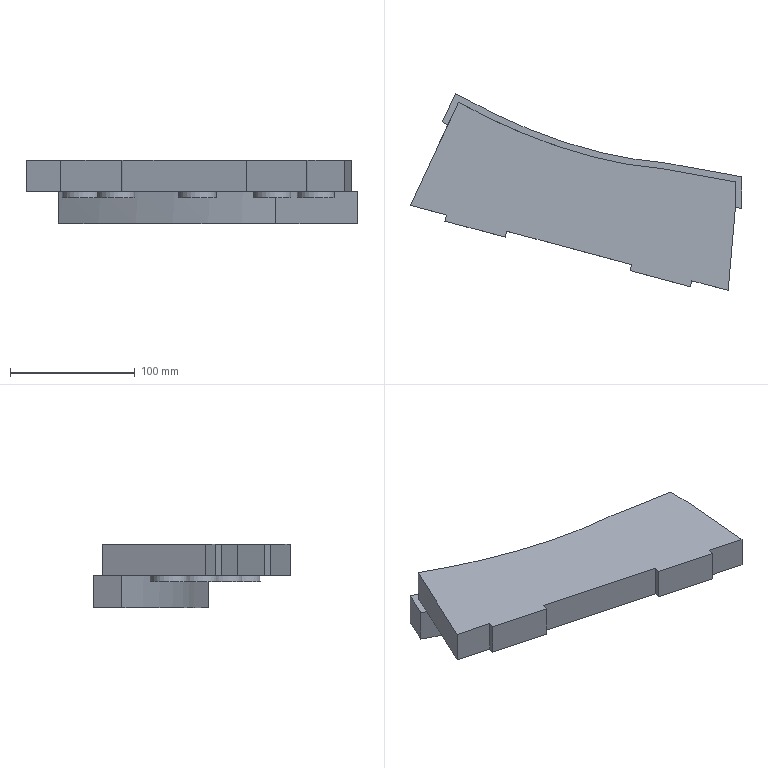Part | NX | features solid 2 | 1 solid | 34 faces | box 265.53 x 157.942 x 51 mm | volume 690173 mm3 | plane 23 | spline 6 | cylinder 5 | commonest cylinder face diameters 30 x5
STEP:
#1=CARTESIAN_POINT('',(-548.514,-260.214,20.));
#2=VERTEX_POINT('',#1);
#3=CARTESIAN_POINT('',(-533.514,-260.214,20.));
#4=DIRECTION('',(0.,0.,-1.));
#5=DIRECTION('',(-1.,0.,0.));
#6=AXIS2_PLACEMENT_3D('',#3,#4,#5);
#7=CIRCLE('',#6,15.);
#8=EDGE_CURVE('',#2,#2,#7,.T.);
#9=ORIENTED_EDGE('',*,*,#8,.T.);
#10=EDGE_LOOP('',(#9));
#11=FACE_BOUND('',#10,.T.);
#12=CARTESIAN_POINT('',(-520.524,-252.714,15.));
#13=VERTEX_POINT('',#12);
#14=CARTESIAN_POINT('',(-533.514,-260.214,15.));
#15=DIRECTION('',(0.,0.,-1.));
#16=DIRECTION('',(0.866,0.5,0.));
#17=AXIS2_PLACEMENT_3D('',#14,#15,#16);
#18=CIRCLE('',#17,15.);
#19=EDGE_CURVE('',#13,#13,#18,.T.);
#20=ORIENTED_EDGE('',*,*,#19,.F.);
#21=EDGE_LOOP('',(#20));
#22=FACE_BOUND('',#21,.T.);
#23=CARTESIAN_POINT('',(-533.514,-260.214,20.));
#24=DIRECTION('',(0.,0.,-1.));
#25=DIRECTION('',(-0.866,-0.5,0.));
#26=AXIS2_PLACEMENT_3D('',#23,#24,#25);
#27=CYLINDRICAL_SURFACE('',#26,15.);
#28=ADVANCED_FACE('',(#11,#22),#27,.T.);
#29=CARTESIAN_POINT('',(-613.514,-240.214,20.));
#30=VERTEX_POINT('',#29);
#31=CARTESIAN_POINT('',(-598.514,-240.214,20.));
#32=DIRECTION('',(0.,0.,-1.));
#33=DIRECTION('',(-1.,0.,0.));
#34=AXIS2_PLACEMENT_3D('',#31,#32,#33);
#35=CIRCLE('',#34,15.);
#36=EDGE_CURVE('',#30,#30,#35,.T.);
#37=ORIENTED_EDGE('',*,*,#36,.T.);
#38=EDGE_LOOP('',(#37));
#39=FACE_BOUND('',#38,.T.);
#40=CARTESIAN_POINT('',(-583.514,-240.214,15.));
#41=VERTEX_POINT('',#40);
#42=CARTESIAN_POINT('',(-598.514,-240.214,15.));
#43=DIRECTION('',(0.,0.,1.));
#44=DIRECTION('',(1.,0.,0.));
#45=AXIS2_PLACEMENT_3D('',#42,#43,#44);
#46=CIRCLE('',#45,15.);
#47=EDGE_CURVE('',#41,#41,#46,.T.);
#48=ORIENTED_EDGE('',*,*,#47,.T.);
#49=EDGE_LOOP('',(#48));
#50=FACE_BOUND('',#49,.T.);
#51=CARTESIAN_POINT('',(-598.514,-240.214,20.));
#52=DIRECTION('',(0.,0.,-1.));
#53=DIRECTION('',(-0.866,-0.5,0.));
#54=AXIS2_PLACEMENT_3D('',#51,#52,#53);
#55=CYLINDRICAL_SURFACE('',#54,15.);
#56=ADVANCED_FACE('',(#39,#50),#55,.T.);
#57=CARTESIAN_POINT('',(-594.55,-271.507,45.));
#58=VERTEX_POINT('',#57);
#59=CARTESIAN_POINT('',(-642.847,-258.566,45.));
#60=VERTEX_POINT('',#59);
#61=CARTESIAN_POINT('',(-576.068,-276.459,45.));
#62=DIRECTION('',(-0.9659,0.2588,0.));
#63=VECTOR('',#62,1000.);
#64=LINE('',#61,#63);
#65=EDGE_CURVE('',#58,#60,#64,.T.);
#66=ORIENTED_EDGE('',*,*,#65,.T.);
#67=CARTESIAN_POINT('',(-642.847,-258.566,20.));
#68=VERTEX_POINT('',#67);
#69=CARTESIAN_POINT('',(-642.847,-258.566,45.));
#70=DIRECTION('',(0.,0.,-1.));
#71=VECTOR('',#70,1000.);
#72=LINE('',#69,#71);
#73=EDGE_CURVE('',#60,#68,#72,.T.);
#74=ORIENTED_EDGE('',*,*,#73,.T.);
#75=CARTESIAN_POINT('',(-594.55,-271.507,20.));
#76=VERTEX_POINT('',#75);
#77=CARTESIAN_POINT('',(-455.717,-308.707,20.));
#78=DIRECTION('',(-0.9659,0.2588,0.));
#79=VECTOR('',#78,1000.);
#80=LINE('',#77,#79);
#81=EDGE_CURVE('',#76,#68,#80,.T.);
#82=ORIENTED_EDGE('',*,*,#81,.F.);
#83=CARTESIAN_POINT('',(-594.55,-271.507,45.));
#84=DIRECTION('',(0.,0.,-1.));
#85=VECTOR('',#84,1000.);
#86=LINE('',#83,#85);
#87=EDGE_CURVE('',#58,#76,#86,.T.);
#88=ORIENTED_EDGE('',*,*,#87,.F.);
#89=EDGE_LOOP('',(#66,#74,#82,#88));
#90=FACE_BOUND('',#89,.T.);
#91=CARTESIAN_POINT('',(-401.118,-323.337,45.));
#92=DIRECTION('',(-0.2588,-0.9659,0.));
#93=DIRECTION('',(0.9659,-0.2588,0.));
#94=AXIS2_PLACEMENT_3D('',#91,#92,#93);
#95=PLANE('',#94);
#96=ADVANCED_FACE('',(#90),#95,.T.);
#97=CARTESIAN_POINT('',(-593.256,-266.677,45.));
#98=VERTEX_POINT('',#97);
#99=CARTESIAN_POINT('',(-593.256,-266.677,20.));
#100=VERTEX_POINT('',#99);
#101=CARTESIAN_POINT('',(-593.256,-266.677,45.));
#102=DIRECTION('',(0.,0.,-1.));
#103=VECTOR('',#102,1000.);
#104=LINE('',#101,#103);
#105=EDGE_CURVE('',#98,#100,#104,.T.);
#106=ORIENTED_EDGE('',*,*,#105,.F.);
#107=CARTESIAN_POINT('',(-594.55,-271.507,45.));
#108=DIRECTION('',(0.2588,0.9659,0.));
#109=VECTOR('',#108,1000.);
#110=LINE('',#107,#109);
#111=EDGE_CURVE('',#58,#98,#110,.T.);
#112=ORIENTED_EDGE('',*,*,#111,.F.);
#113=ORIENTED_EDGE('',*,*,#87,.T.);
#114=CARTESIAN_POINT('',(-594.55,-271.507,20.));
#115=DIRECTION('',(0.2588,0.9659,0.));
#116=VECTOR('',#115,1000.);
#117=LINE('',#114,#116);
#118=EDGE_CURVE('',#76,#100,#117,.T.);
#119=ORIENTED_EDGE('',*,*,#118,.T.);
#120=EDGE_LOOP('',(#106,#112,#113,#119));
#121=FACE_BOUND('',#120,.T.);
#122=CARTESIAN_POINT('',(-594.55,-271.507,45.));
#123=DIRECTION('',(0.9659,-0.2588,0.));
#124=DIRECTION('',(0.2588,0.9659,0.));
#125=AXIS2_PLACEMENT_3D('',#122,#123,#124);
#126=PLANE('',#125);
#127=ADVANCED_FACE('',(#121),#126,.T.);
#128=CARTESIAN_POINT('',(-641.553,-253.736,45.));
#129=VERTEX_POINT('',#128);
#130=CARTESIAN_POINT('',(-670.53,-245.972,45.));
#131=VERTEX_POINT('',#130);
#132=CARTESIAN_POINT('',(-574.774,-271.63,45.));
#133=DIRECTION('',(-0.9659,0.2588,0.));
#134=VECTOR('',#133,1000.);
#135=LINE('',#132,#134);
#136=EDGE_CURVE('',#129,#131,#135,.T.);
#137=ORIENTED_EDGE('',*,*,#136,.T.);
#138=CARTESIAN_POINT('',(-670.53,-245.972,20.));
#139=VERTEX_POINT('',#138);
#140=CARTESIAN_POINT('',(-670.53,-245.972,45.));
#141=DIRECTION('',(0.,0.,-1.));
#142=VECTOR('',#141,1000.);
#143=LINE('',#140,#142);
#144=EDGE_CURVE('',#131,#139,#143,.T.);
#145=ORIENTED_EDGE('',*,*,#144,.T.);
#146=CARTESIAN_POINT('',(-641.553,-253.736,20.));
#147=VERTEX_POINT('',#146);
#148=CARTESIAN_POINT('',(-454.423,-303.878,20.));
#149=DIRECTION('',(-0.9659,0.2588,0.));
#150=VECTOR('',#149,1000.);
#151=LINE('',#148,#150);
#152=EDGE_CURVE('',#147,#139,#151,.T.);
#153=ORIENTED_EDGE('',*,*,#152,.F.);
#154=CARTESIAN_POINT('',(-641.553,-253.736,45.));
#155=DIRECTION('',(0.,0.,-1.));
#156=VECTOR('',#155,1000.);
#157=LINE('',#154,#156);
#158=EDGE_CURVE('',#129,#147,#157,.T.);
#159=ORIENTED_EDGE('',*,*,#158,.F.);
#160=EDGE_LOOP('',(#137,#145,#153,#159));
#161=FACE_BOUND('',#160,.T.);
#162=CARTESIAN_POINT('',(-399.824,-318.507,45.));
#163=DIRECTION('',(-0.2588,-0.9659,0.));
#164=DIRECTION('',(0.9659,-0.2588,0.));
#165=AXIS2_PLACEMENT_3D('',#162,#163,#164);
#166=PLANE('',#165);
#167=ADVANCED_FACE('',(#161),#166,.T.);
#168=ORIENTED_EDGE('',*,*,#158,.T.);
#169=CARTESIAN_POINT('',(-642.847,-258.566,20.));
#170=DIRECTION('',(0.2588,0.9659,0.));
#171=VECTOR('',#170,1000.);
#172=LINE('',#169,#171);
#173=EDGE_CURVE('',#68,#147,#172,.T.);
#174=ORIENTED_EDGE('',*,*,#173,.F.);
#175=ORIENTED_EDGE('',*,*,#73,.F.);
#176=CARTESIAN_POINT('',(-642.847,-258.566,45.));
#177=DIRECTION('',(0.2588,0.9659,0.));
#178=VECTOR('',#177,1000.);
#179=LINE('',#176,#178);
#180=EDGE_CURVE('',#60,#129,#179,.T.);
#181=ORIENTED_EDGE('',*,*,#180,.T.);
#182=EDGE_LOOP('',(#168,#174,#175,#181));
#183=FACE_BOUND('',#182,.T.);
#184=CARTESIAN_POINT('',(-642.847,-258.566,45.));
#185=DIRECTION('',(0.9659,-0.2588,0.));
#186=DIRECTION('',(0.2588,0.9659,0.));
#187=AXIS2_PLACEMENT_3D('',#184,#185,#186);
#188=PLANE('',#187);
#189=ADVANCED_FACE('',(#183),#188,.F.);
#190=CARTESIAN_POINT('',(-425.524,-262.714,15.));
#191=VERTEX_POINT('',#190);
#192=CARTESIAN_POINT('',(-438.514,-270.214,15.));
#193=DIRECTION('',(0.,0.,-1.));
#194=DIRECTION('',(0.866,0.5,0.));
#195=AXIS2_PLACEMENT_3D('',#192,#193,#194);
#196=CIRCLE('',#195,15.);
#197=EDGE_CURVE('',#191,#191,#196,.T.);
#198=ORIENTED_EDGE('',*,*,#197,.F.);
#199=EDGE_LOOP('',(#198));
#200=FACE_BOUND('',#199,.T.);
#201=CARTESIAN_POINT('',(-453.514,-270.214,20.));
#202=VERTEX_POINT('',#201);
#203=CARTESIAN_POINT('',(-438.514,-270.214,20.));
#204=DIRECTION('',(0.,0.,-1.));
#205=DIRECTION('',(-1.,0.,0.));
#206=AXIS2_PLACEMENT_3D('',#203,#204,#205);
#207=CIRCLE('',#206,15.);
#208=EDGE_CURVE('',#202,#202,#207,.T.);
#209=ORIENTED_EDGE('',*,*,#208,.T.);
#210=EDGE_LOOP('',(#209));
#211=FACE_BOUND('',#210,.T.);
#212=CARTESIAN_POINT('',(-438.514,-270.214,20.));
#213=DIRECTION('',(0.,0.,-1.));
#214=DIRECTION('',(-0.866,-0.5,0.));
#215=AXIS2_PLACEMENT_3D('',#212,#213,#214);
#216=CYLINDRICAL_SURFACE('',#215,15.);
#217=ADVANCED_FACE('',(#200,#211),#216,.T.);
#218=CARTESIAN_POINT('',(-415.836,-314.217,20.));
#219=VERTEX_POINT('',#218);
#220=CARTESIAN_POINT('',(-410.,-247.512,20.));
#221=VERTEX_POINT('',#220);
#222=CARTESIAN_POINT('',(-409.784,-245.039,20.));
#223=DIRECTION('',(0.08716,0.9962,0.));
#224=VECTOR('',#223,1000.);
#225=LINE('',#222,#224);
#226=EDGE_CURVE('',#219,#221,#225,.T.);
#227=ORIENTED_EDGE('',*,*,#226,.T.);
#228=CARTESIAN_POINT('',(-410.,-247.512,45.));
#229=VERTEX_POINT('',#228);
#230=CARTESIAN_POINT('',(-410.,-247.512,20.));
#231=DIRECTION('',(0.,0.,1.));
#232=VECTOR('',#231,1000.);
#233=LINE('',#230,#232);
#234=EDGE_CURVE('',#221,#229,#233,.T.);
#235=ORIENTED_EDGE('',*,*,#234,.T.);
#236=CARTESIAN_POINT('',(-415.836,-314.217,45.));
#237=VERTEX_POINT('',#236);
#238=CARTESIAN_POINT('',(-406.364,-205.947,45.));
#239=DIRECTION('',(0.08716,0.9962,0.));
#240=VECTOR('',#239,1000.);
#241=LINE('',#238,#240);
#242=EDGE_CURVE('',#237,#229,#241,.T.);
#243=ORIENTED_EDGE('',*,*,#242,.F.);
#244=CARTESIAN_POINT('',(-415.836,-314.217,45.));
#245=DIRECTION('',(0.,0.,-1.));
#246=VECTOR('',#245,1000.);
#247=LINE('',#244,#246);
#248=EDGE_CURVE('',#237,#219,#247,.T.);
#249=ORIENTED_EDGE('',*,*,#248,.T.);
#250=EDGE_LOOP('',(#227,#235,#243,#249));
#251=FACE_BOUND('',#250,.T.);
#252=CARTESIAN_POINT('',(-410.,-247.512,26.));
#253=DIRECTION('',(-0.9962,0.08716,0.));
#254=DIRECTION('',(-0.08716,-0.9962,0.));
#255=AXIS2_PLACEMENT_3D('',#252,#253,#254);
#256=PLANE('',#255);
#257=ADVANCED_FACE('',(#251),#256,.F.);
#258=CARTESIAN_POINT('',(-640.447,-181.458,20.));
#259=VERTEX_POINT('',#258);
#260=CARTESIAN_POINT('',(-470.646,-236.588,20.));
#261=VERTEX_POINT('',#260);
#262=CARTESIAN_POINT('',(-640.447,-181.458,20.));
#263=CARTESIAN_POINT('',(-627.329,-188.713,20.));
#264=CARTESIAN_POINT('',(-600.49,-202.118,20.));
#265=CARTESIAN_POINT('',(-558.614,-218.615,20.));
#266=CARTESIAN_POINT('',(-515.266,-230.753,20.));
#267=CARTESIAN_POINT('',(-485.578,-235.315,20.));
#268=CARTESIAN_POINT('',(-470.646,-236.588,20.));
#269=B_SPLINE_CURVE_WITH_KNOTS('',3,(#262,#263,#264,#265,#266,#267,#268),.UNSPECIFIED.,.F.,.F.,(4,1,1,1,4),(0.7368,0.7817,0.8267,0.8717,0.9167),.UNSPECIFIED.);
#270=EDGE_CURVE('',#259,#261,#269,.T.);
#271=ORIENTED_EDGE('',*,*,#270,.F.);
#272=CARTESIAN_POINT('',(-644.823,-179.011,20.));
#273=VERTEX_POINT('',#272);
#274=CARTESIAN_POINT('',(-644.823,-179.011,20.));
#275=CARTESIAN_POINT('',(-643.368,-179.833,20.));
#276=CARTESIAN_POINT('',(-641.909,-180.649,20.));
#277=CARTESIAN_POINT('',(-640.447,-181.458,20.));
#278=B_SPLINE_CURVE_WITH_KNOTS('',3,(#274,#275,#276,#277),.UNSPECIFIED.,.F.,.F.,(4,4),(0.7318,0.7368),.UNSPECIFIED.);
#279=EDGE_CURVE('',#273,#259,#278,.T.);
#280=ORIENTED_EDGE('',*,*,#279,.F.);
#281=CARTESIAN_POINT('',(-644.823,-179.011,-6.));
#282=VERTEX_POINT('',#281);
#283=CARTESIAN_POINT('',(-644.823,-179.011,45.));
#284=DIRECTION('',(0.,0.,-1.));
#285=VECTOR('',#284,1000.);
#286=LINE('',#283,#285);
#287=EDGE_CURVE('',#273,#282,#286,.T.);
#288=ORIENTED_EDGE('',*,*,#287,.T.);
#289=CARTESIAN_POINT('',(-470.646,-236.588,-6.));
#290=VERTEX_POINT('',#289);
#291=CARTESIAN_POINT('',(-644.823,-179.011,-6.));
#292=CARTESIAN_POINT('',(-641.958,-180.631,-6.));
#293=CARTESIAN_POINT('',(-622.134,-191.596,-6.));
#294=CARTESIAN_POINT('',(-584.151,-209.58,-6.));
#295=CARTESIAN_POINT('',(-528.839,-228.144,-6.));
#296=CARTESIAN_POINT('',(-490.07,-234.932,-6.));
#297=CARTESIAN_POINT('',(-470.646,-236.588,-6.));
#298=B_SPLINE_CURVE_WITH_KNOTS('',3,(#291,#292,#293,#294,#295,#296,#297),.UNSPECIFIED.,.F.,.F.,(4,1,1,1,4),(0.,0.04001,0.2754,0.5108,0.7411),.UNSPECIFIED.);
#299=EDGE_CURVE('',#282,#290,#298,.T.);
#300=ORIENTED_EDGE('',*,*,#299,.T.);
#301=CARTESIAN_POINT('',(-470.646,-236.588,45.));
#302=DIRECTION('',(0.,0.,-1.));
#303=VECTOR('',#302,1000.);
#304=LINE('',#301,#303);
#305=EDGE_CURVE('',#261,#290,#304,.T.);
#306=ORIENTED_EDGE('',*,*,#305,.F.);
#307=EDGE_LOOP('',(#271,#280,#288,#300,#306));
#308=FACE_BOUND('',#307,.T.);
#309=CARTESIAN_POINT('',(-644.823,-179.011,20.));
#310=CARTESIAN_POINT('',(-644.823,-179.011,-6.));
#311=CARTESIAN_POINT('',(-631.553,-186.516,20.));
#312=CARTESIAN_POINT('',(-631.553,-186.516,-6.));
#313=CARTESIAN_POINT('',(-604.421,-200.366,20.));
#314=CARTESIAN_POINT('',(-604.421,-200.366,-6.));
#315=CARTESIAN_POINT('',(-561.818,-217.552,20.));
#316=CARTESIAN_POINT('',(-561.818,-217.552,-6.));
#317=CARTESIAN_POINT('',(-517.207,-230.394,20.));
#318=CARTESIAN_POINT('',(-517.207,-230.394,-6.));
#319=CARTESIAN_POINT('',(-486.272,-235.255,20.));
#320=CARTESIAN_POINT('',(-486.272,-235.255,-6.));
#321=CARTESIAN_POINT('',(-470.646,-236.588,20.));
#322=CARTESIAN_POINT('',(-470.646,-236.588,-6.));
#323=B_SPLINE_SURFACE_WITH_KNOTS('',3,1,((#309,#310),(#311,#312),(#313,#314),(#315,#316),(#317,#318),(#319,#320),(#321,#322)),.SURF_OF_LINEAR_EXTRUSION.,.F.,.F.,.F.,(4,1,1,1,4),(2,2),(0.,0.1853,0.3706,0.5559,0.7411),(0.,1.),.UNSPECIFIED.);
#324=ADVANCED_FACE('',(#308),#323,.F.);
#325=CARTESIAN_POINT('',(-405.,-248.354,-6.));
#326=VERTEX_POINT('',#325);
#327=CARTESIAN_POINT('',(-470.646,-236.588,-6.));
#328=CARTESIAN_POINT('',(-456.993,-239.107,-6.));
#329=CARTESIAN_POINT('',(-435.255,-243.115,-6.));
#330=CARTESIAN_POINT('',(-413.219,-246.983,-6.));
#331=CARTESIAN_POINT('',(-405.,-248.354,-6.));
#332=B_SPLINE_CURVE_WITH_KNOTS('',3,(#327,#328,#329,#330,#331),.UNSPECIFIED.,.F.,.F.,(4,1,4),(0.7411,0.9039,1.),.UNSPECIFIED.);
#333=EDGE_CURVE('',#290,#326,#332,.T.);
#334=ORIENTED_EDGE('',*,*,#333,.T.);
#335=CARTESIAN_POINT('',(-405.,-248.354,20.));
#336=VERTEX_POINT('',#335);
#337=CARTESIAN_POINT('',(-405.,-248.354,45.));
#338=DIRECTION('',(0.,0.,-1.));
#339=VECTOR('',#338,1000.);
#340=LINE('',#337,#339);
#341=EDGE_CURVE('',#336,#326,#340,.T.);
#342=ORIENTED_EDGE('',*,*,#341,.F.);
#343=CARTESIAN_POINT('',(-470.646,-236.588,20.));
#344=CARTESIAN_POINT('',(-456.993,-239.107,20.));
#345=CARTESIAN_POINT('',(-435.255,-243.115,20.));
#346=CARTESIAN_POINT('',(-413.219,-246.983,20.));
#347=CARTESIAN_POINT('',(-405.,-248.354,20.));
#348=B_SPLINE_CURVE_WITH_KNOTS('',3,(#343,#344,#345,#346,#347),.UNSPECIFIED.,.F.,.F.,(4,1,4),(0.7411,0.9039,1.),.UNSPECIFIED.);
#349=EDGE_CURVE('',#336,#221,#348,.F.);
#350=ORIENTED_EDGE('',*,*,#349,.T.);
#351=CARTESIAN_POINT('',(-470.646,-236.588,20.));
#352=CARTESIAN_POINT('',(-450.446,-240.315,20.));
#353=CARTESIAN_POINT('',(-430.25,-244.067,20.));
#354=CARTESIAN_POINT('',(-410.,-247.512,20.));
#355=B_SPLINE_CURVE_WITH_KNOTS('',3,(#351,#352,#353,#354),.UNSPECIFIED.,.F.,.F.,(4,4),(0.07034,0.132),.UNSPECIFIED.);
#356=EDGE_CURVE('',#261,#221,#355,.T.);
#357=ORIENTED_EDGE('',*,*,#356,.F.);
#358=ORIENTED_EDGE('',*,*,#305,.T.);
#359=EDGE_LOOP('',(#334,#342,#350,#357,#358));
#360=FACE_BOUND('',#359,.T.);
#361=CARTESIAN_POINT('',(-470.646,-236.588,20.));
#362=CARTESIAN_POINT('',(-470.646,-236.588,-6.));
#363=CARTESIAN_POINT('',(-448.934,-240.594,20.));
#364=CARTESIAN_POINT('',(-448.934,-240.594,-6.));
#365=CARTESIAN_POINT('',(-427.143,-244.66,20.));
#366=CARTESIAN_POINT('',(-427.143,-244.66,-6.));
#367=CARTESIAN_POINT('',(-405.,-248.354,20.));
#368=CARTESIAN_POINT('',(-405.,-248.354,-6.));
#369=B_SPLINE_SURFACE_WITH_KNOTS('',3,1,((#361,#362),(#363,#364),(#365,#366),(#367,#368)),.SURF_OF_LINEAR_EXTRUSION.,.F.,.F.,.F.,(4,4),(2,2),(0.7411,1.),(0.,1.),.PIECEWISE_BEZIER_KNOTS.);
#370=ADVANCED_FACE('',(#360),#369,.F.);
#371=CARTESIAN_POINT('',(-613.873,-209.233,15.));
#372=VERTEX_POINT('',#371);
#373=CARTESIAN_POINT('',(-626.864,-216.733,15.));
#374=DIRECTION('',(0.,0.,-1.));
#375=DIRECTION('',(0.866,0.5,0.));
#376=AXIS2_PLACEMENT_3D('',#373,#374,#375);
#377=CIRCLE('',#376,15.);
#378=EDGE_CURVE('',#372,#372,#377,.T.);
#379=ORIENTED_EDGE('',*,*,#378,.F.);
#380=EDGE_LOOP('',(#379));
#381=FACE_BOUND('',#380,.T.);
#382=CARTESIAN_POINT('',(-641.864,-216.733,20.));
#383=VERTEX_POINT('',#382);
#384=CARTESIAN_POINT('',(-626.864,-216.733,20.));
#385=DIRECTION('',(0.,0.,-1.));
#386=DIRECTION('',(-1.,0.,0.));
#387=AXIS2_PLACEMENT_3D('',#384,#385,#386);
#388=CIRCLE('',#387,15.);
#389=EDGE_CURVE('',#383,#383,#388,.T.);
#390=ORIENTED_EDGE('',*,*,#389,.T.);
#391=EDGE_LOOP('',(#390));
#392=FACE_BOUND('',#391,.T.);
#393=CARTESIAN_POINT('',(-626.864,-216.733,20.));
#394=DIRECTION('',(0.,0.,-1.));
#395=DIRECTION('',(-0.866,-0.5,0.));
#396=AXIS2_PLACEMENT_3D('',#393,#394,#395);
#397=CYLINDRICAL_SURFACE('',#396,15.);
#398=ADVANCED_FACE('',(#381,#392),#397,.T.);
#399=CARTESIAN_POINT('',(-488.514,-275.214,20.));
#400=VERTEX_POINT('',#399);
#401=CARTESIAN_POINT('',(-473.514,-275.214,20.));
#402=DIRECTION('',(0.,0.,-1.));
#403=DIRECTION('',(-1.,0.,0.));
#404=AXIS2_PLACEMENT_3D('',#401,#402,#403);
#405=CIRCLE('',#404,15.);
#406=EDGE_CURVE('',#400,#400,#405,.T.);
#407=ORIENTED_EDGE('',*,*,#406,.T.);
#408=EDGE_LOOP('',(#407));
#409=FACE_BOUND('',#408,.T.);
#410=CARTESIAN_POINT('',(-460.524,-267.714,15.));
#411=VERTEX_POINT('',#410);
#412=CARTESIAN_POINT('',(-473.514,-275.214,15.));
#413=DIRECTION('',(0.,0.,-1.));
#414=DIRECTION('',(0.866,0.5,0.));
#415=AXIS2_PLACEMENT_3D('',#412,#413,#414);
#416=CIRCLE('',#415,15.);
#417=EDGE_CURVE('',#411,#411,#416,.T.);
#418=ORIENTED_EDGE('',*,*,#417,.F.);
#419=EDGE_LOOP('',(#418));
#420=FACE_BOUND('',#419,.T.);
#421=CARTESIAN_POINT('',(-473.514,-275.214,20.));
#422=DIRECTION('',(0.,0.,-1.));
#423=DIRECTION('',(-0.866,-0.5,0.));
#424=AXIS2_PLACEMENT_3D('',#421,#422,#423);
#425=CYLINDRICAL_SURFACE('',#424,15.);
#426=ADVANCED_FACE('',(#409,#420),#425,.T.);
#427=CARTESIAN_POINT('',(-446.108,-311.282,45.));
#428=VERTEX_POINT('',#427);
#429=CARTESIAN_POINT('',(-494.404,-298.341,45.));
#430=VERTEX_POINT('',#429);
#431=CARTESIAN_POINT('',(-398.648,-323.999,45.));
#432=DIRECTION('',(-0.9659,0.2588,0.));
#433=VECTOR('',#432,1000.);
#434=LINE('',#431,#433);
#435=EDGE_CURVE('',#428,#430,#434,.T.);
#436=ORIENTED_EDGE('',*,*,#435,.T.);
#437=CARTESIAN_POINT('',(-494.404,-298.341,20.));
#438=VERTEX_POINT('',#437);
#439=CARTESIAN_POINT('',(-494.404,-298.341,45.));
#440=DIRECTION('',(0.,0.,-1.));
#441=VECTOR('',#440,1000.);
#442=LINE('',#439,#441);
#443=EDGE_CURVE('',#430,#438,#442,.T.);
#444=ORIENTED_EDGE('',*,*,#443,.T.);
#445=CARTESIAN_POINT('',(-446.108,-311.282,20.));
#446=VERTEX_POINT('',#445);
#447=CARTESIAN_POINT('',(-278.297,-356.247,20.));
#448=DIRECTION('',(-0.9659,0.2588,0.));
#449=VECTOR('',#448,1000.);
#450=LINE('',#447,#449);
#451=EDGE_CURVE('',#446,#438,#450,.T.);
#452=ORIENTED_EDGE('',*,*,#451,.F.);
#453=CARTESIAN_POINT('',(-446.108,-311.282,45.));
#454=DIRECTION('',(0.,0.,-1.));
#455=VECTOR('',#454,1000.);
#456=LINE('',#453,#455);
#457=EDGE_CURVE('',#428,#446,#456,.T.);
#458=ORIENTED_EDGE('',*,*,#457,.F.);
#459=EDGE_LOOP('',(#436,#444,#452,#458));
#460=FACE_BOUND('',#459,.T.);
#461=CARTESIAN_POINT('',(-223.697,-370.877,45.));
#462=DIRECTION('',(-0.2588,-0.9659,0.));
#463=DIRECTION('',(0.9659,-0.2588,0.));
#464=AXIS2_PLACEMENT_3D('',#461,#462,#463);
#465=PLANE('',#464);
#466=ADVANCED_FACE('',(#460),#465,.T.);
#467=CARTESIAN_POINT('',(-444.814,-306.452,45.));
#468=VERTEX_POINT('',#467);
#469=CARTESIAN_POINT('',(-444.814,-306.452,20.));
#470=VERTEX_POINT('',#469);
#471=CARTESIAN_POINT('',(-444.814,-306.452,45.));
#472=DIRECTION('',(0.,0.,-1.));
#473=VECTOR('',#472,1000.);
#474=LINE('',#471,#473);
#475=EDGE_CURVE('',#468,#470,#474,.T.);
#476=ORIENTED_EDGE('',*,*,#475,.F.);
#477=CARTESIAN_POINT('',(-446.108,-311.282,45.));
#478=DIRECTION('',(0.2588,0.9659,0.));
#479=VECTOR('',#478,1000.);
#480=LINE('',#477,#479);
#481=EDGE_CURVE('',#428,#468,#480,.T.);
#482=ORIENTED_EDGE('',*,*,#481,.F.);
#483=ORIENTED_EDGE('',*,*,#457,.T.);
#484=CARTESIAN_POINT('',(-446.108,-311.282,20.));
#485=DIRECTION('',(0.2588,0.9659,0.));
#486=VECTOR('',#485,1000.);
#487=LINE('',#484,#486);
#488=EDGE_CURVE('',#446,#470,#487,.T.);
#489=ORIENTED_EDGE('',*,*,#488,.T.);
#490=EDGE_LOOP('',(#476,#482,#483,#489));
#491=FACE_BOUND('',#490,.T.);
#492=CARTESIAN_POINT('',(-446.108,-311.282,45.));
#493=DIRECTION('',(0.9659,-0.2588,0.));
#494=DIRECTION('',(0.2588,0.9659,0.));
#495=AXIS2_PLACEMENT_3D('',#492,#493,#494);
#496=PLANE('',#495);
#497=ADVANCED_FACE('',(#491),#496,.T.);
#498=CARTESIAN_POINT('',(-493.11,-293.511,45.));
#499=VERTEX_POINT('',#498);
#500=CARTESIAN_POINT('',(-493.11,-293.511,20.));
#501=VERTEX_POINT('',#500);
#502=CARTESIAN_POINT('',(-493.11,-293.511,45.));
#503=DIRECTION('',(0.,0.,-1.));
#504=VECTOR('',#503,1000.);
#505=LINE('',#502,#504);
#506=EDGE_CURVE('',#499,#501,#505,.T.);
#507=ORIENTED_EDGE('',*,*,#506,.T.);
#508=CARTESIAN_POINT('',(-494.404,-298.341,20.));
#509=DIRECTION('',(0.2588,0.9659,0.));
#510=VECTOR('',#509,1000.);
#511=LINE('',#508,#510);
#512=EDGE_CURVE('',#438,#501,#511,.T.);
#513=ORIENTED_EDGE('',*,*,#512,.F.);
#514=ORIENTED_EDGE('',*,*,#443,.F.);
#515=CARTESIAN_POINT('',(-494.404,-298.341,45.));
#516=DIRECTION('',(0.2588,0.9659,0.));
#517=VECTOR('',#516,1000.);
#518=LINE('',#515,#517);
#519=EDGE_CURVE('',#430,#499,#518,.T.);
#520=ORIENTED_EDGE('',*,*,#519,.T.);
#521=EDGE_LOOP('',(#507,#513,#514,#520));
#522=FACE_BOUND('',#521,.T.);
#523=CARTESIAN_POINT('',(-494.404,-298.341,45.));
#524=DIRECTION('',(0.9659,-0.2588,0.));
#525=DIRECTION('',(0.2588,0.9659,0.));
#526=AXIS2_PLACEMENT_3D('',#523,#524,#525);
#527=PLANE('',#526);
#528=ADVANCED_FACE('',(#522),#527,.F.);
#529=ORIENTED_EDGE('',*,*,#475,.T.);
#530=CARTESIAN_POINT('',(-454.423,-303.878,20.));
#531=DIRECTION('',(-0.9659,0.2588,0.));
#532=VECTOR('',#531,1000.);
#533=LINE('',#530,#532);
#534=EDGE_CURVE('',#219,#470,#533,.T.);
#535=ORIENTED_EDGE('',*,*,#534,.F.);
#536=ORIENTED_EDGE('',*,*,#248,.F.);
#537=CARTESIAN_POINT('',(-574.774,-271.63,45.));
#538=DIRECTION('',(-0.9659,0.2588,0.));
#539=VECTOR('',#538,1000.);
#540=LINE('',#537,#539);
#541=EDGE_CURVE('',#237,#468,#540,.T.);
#542=ORIENTED_EDGE('',*,*,#541,.T.);
#543=EDGE_LOOP('',(#529,#535,#536,#542));
#544=FACE_BOUND('',#543,.T.);
#545=CARTESIAN_POINT('',(-399.824,-318.507,45.));
#546=DIRECTION('',(-0.2588,-0.9659,0.));
#547=DIRECTION('',(0.9659,-0.2588,0.));
#548=AXIS2_PLACEMENT_3D('',#545,#546,#547);
#549=PLANE('',#548);
#550=ADVANCED_FACE('',(#544),#549,.T.);
#551=CARTESIAN_POINT('',(-454.423,-303.878,20.));
#552=DIRECTION('',(-0.9659,0.2588,0.));
#553=VECTOR('',#552,1000.);
#554=LINE('',#551,#553);
#555=EDGE_CURVE('',#501,#100,#554,.T.);
#556=ORIENTED_EDGE('',*,*,#555,.F.);
#557=ORIENTED_EDGE('',*,*,#506,.F.);
#558=CARTESIAN_POINT('',(-574.774,-271.63,45.));
#559=DIRECTION('',(-0.9659,0.2588,0.));
#560=VECTOR('',#559,1000.);
#561=LINE('',#558,#560);
#562=EDGE_CURVE('',#499,#98,#561,.T.);
#563=ORIENTED_EDGE('',*,*,#562,.T.);
#564=ORIENTED_EDGE('',*,*,#105,.T.);
#565=EDGE_LOOP('',(#556,#557,#563,#564));
#566=FACE_BOUND('',#565,.T.);
#567=CARTESIAN_POINT('',(-399.824,-318.507,45.));
#568=DIRECTION('',(-0.2588,-0.9659,0.));
#569=DIRECTION('',(0.9659,-0.2588,0.));
#570=AXIS2_PLACEMENT_3D('',#567,#568,#569);
#571=PLANE('',#570);
#572=ADVANCED_FACE('',(#566),#571,.T.);
#573=ORIENTED_EDGE('',*,*,#299,.F.);
#574=CARTESIAN_POINT('',(-634.221,-156.275,-6.));
#575=VERTEX_POINT('',#574);
#576=CARTESIAN_POINT('',(-634.221,-156.275,-6.));
#577=DIRECTION('',(-0.4226,-0.9063,0.));
#578=VECTOR('',#577,1000.);
#579=LINE('',#576,#578);
#580=EDGE_CURVE('',#575,#282,#579,.T.);
#581=ORIENTED_EDGE('',*,*,#580,.F.);
#582=CARTESIAN_POINT('',(-467.332,-211.778,-6.));
#583=VERTEX_POINT('',#582);
#584=CARTESIAN_POINT('',(-634.221,-156.275,-6.));
#585=CARTESIAN_POINT('',(-625.502,-161.258,-6.));
#586=CARTESIAN_POINT('',(-602.187,-173.648,-6.));
#587=CARTESIAN_POINT('',(-562.946,-190.715,-6.));
#588=CARTESIAN_POINT('',(-515.99,-205.204,-6.));
#589=CARTESIAN_POINT('',(-483.626,-210.452,-6.));
#590=CARTESIAN_POINT('',(-467.332,-211.778,-6.));
#591=B_SPLINE_CURVE_WITH_KNOTS('',3,(#584,#585,#586,#587,#588,#589,#590),.UNSPECIFIED.,.F.,.F.,(4,1,1,1,4),(0.,0.1252,0.3291,0.5329,0.7368),.UNSPECIFIED.);
#592=EDGE_CURVE('',#575,#583,#591,.T.);
#593=ORIENTED_EDGE('',*,*,#592,.T.);
#594=CARTESIAN_POINT('',(-405.,-223.005,-6.));
#595=VERTEX_POINT('',#594);
#596=CARTESIAN_POINT('',(-467.332,-211.778,-6.));
#597=CARTESIAN_POINT('',(-453.683,-214.296,-6.));
#598=CARTESIAN_POINT('',(-432.922,-218.124,-6.));
#599=CARTESIAN_POINT('',(-412.13,-221.796,-6.));
#600=CARTESIAN_POINT('',(-405.,-223.005,-6.));
#601=B_SPLINE_CURVE_WITH_KNOTS('',3,(#596,#597,#598,#599,#600),.UNSPECIFIED.,.F.,.F.,(4,1,4),(0.7368,0.9098,1.),.UNSPECIFIED.);
#602=EDGE_CURVE('',#583,#595,#601,.T.);
#603=ORIENTED_EDGE('',*,*,#602,.T.);
#604=CARTESIAN_POINT('',(-405.,-1052.635,-6.));
#605=DIRECTION('',(0.,1.,0.));
#606=VECTOR('',#605,1000.);
#607=LINE('',#604,#606);
#608=EDGE_CURVE('',#326,#595,#607,.T.);
#609=ORIENTED_EDGE('',*,*,#608,.F.);
#610=ORIENTED_EDGE('',*,*,#333,.F.);
#611=EDGE_LOOP('',(#573,#581,#593,#603,#609,#610));
#612=FACE_BOUND('',#611,.T.);
#613=CARTESIAN_POINT('',(-918.37,-664.302,-6.));
#614=DIRECTION('',(0.,0.,1.));
#615=DIRECTION('',(1.,0.,0.));
#616=AXIS2_PLACEMENT_3D('',#613,#614,#615);
#617=PLANE('',#616);
#618=ADVANCED_FACE('',(#612),#617,.F.);
#619=CARTESIAN_POINT('',(-405.,-223.005,20.));
#620=VERTEX_POINT('',#619);
#621=CARTESIAN_POINT('',(-405.,-401.561,20.));
#622=DIRECTION('',(0.,1.,0.));
#623=VECTOR('',#622,1000.);
#624=LINE('',#621,#623);
#625=EDGE_CURVE('',#620,#336,#624,.F.);
#626=ORIENTED_EDGE('',*,*,#625,.F.);
#627=CARTESIAN_POINT('',(-467.332,-211.778,20.));
#628=VERTEX_POINT('',#627);
#629=CARTESIAN_POINT('',(-467.332,-211.778,20.));
#630=CARTESIAN_POINT('',(-453.683,-214.296,20.));
#631=CARTESIAN_POINT('',(-432.922,-218.124,20.));
#632=CARTESIAN_POINT('',(-412.13,-221.796,20.));
#633=CARTESIAN_POINT('',(-405.,-223.005,20.));
#634=B_SPLINE_CURVE_WITH_KNOTS('',3,(#629,#630,#631,#632,#633),.UNSPECIFIED.,.F.,.F.,(4,1,4),(0.7368,0.9098,1.),.UNSPECIFIED.);
#635=EDGE_CURVE('',#620,#628,#634,.F.);
#636=ORIENTED_EDGE('',*,*,#635,.T.);
#637=CARTESIAN_POINT('',(-634.221,-156.275,20.));
#638=VERTEX_POINT('',#637);
#639=CARTESIAN_POINT('',(-634.221,-156.275,20.));
#640=CARTESIAN_POINT('',(-625.502,-161.258,20.));
#641=CARTESIAN_POINT('',(-602.187,-173.648,20.));
#642=CARTESIAN_POINT('',(-562.946,-190.715,20.));
#643=CARTESIAN_POINT('',(-515.99,-205.204,20.));
#644=CARTESIAN_POINT('',(-483.626,-210.452,20.));
#645=CARTESIAN_POINT('',(-467.332,-211.778,20.));
#646=B_SPLINE_CURVE_WITH_KNOTS('',3,(#639,#640,#641,#642,#643,#644,#645),.UNSPECIFIED.,.F.,.F.,(4,1,1,1,4),(0.,0.1252,0.3291,0.5329,0.7368),.UNSPECIFIED.);
#647=EDGE_CURVE('',#628,#638,#646,.F.);
#648=ORIENTED_EDGE('',*,*,#647,.T.);
#649=CARTESIAN_POINT('',(-634.221,-156.275,20.));
#650=DIRECTION('',(0.4226,0.9063,0.));
#651=VECTOR('',#650,1000.);
#652=LINE('',#649,#651);
#653=EDGE_CURVE('',#273,#638,#652,.T.);
#654=ORIENTED_EDGE('',*,*,#653,.F.);
#655=ORIENTED_EDGE('',*,*,#279,.T.);
#656=CARTESIAN_POINT('',(-631.973,-163.285,20.));
#657=VERTEX_POINT('',#656);
#658=CARTESIAN_POINT('',(-629.689,-158.388,20.));
#659=DIRECTION('',(-0.4226,-0.9063,0.));
#660=VECTOR('',#659,1000.);
#661=LINE('',#658,#660);
#662=EDGE_CURVE('',#657,#259,#661,.T.);
#663=ORIENTED_EDGE('',*,*,#662,.F.);
#664=CARTESIAN_POINT('',(-467.991,-216.741,20.));
#665=VERTEX_POINT('',#664);
#666=CARTESIAN_POINT('',(-631.973,-163.285,20.));
#667=CARTESIAN_POINT('',(-619.351,-170.317,20.));
#668=CARTESIAN_POINT('',(-593.517,-183.297,20.));
#669=CARTESIAN_POINT('',(-553.157,-199.317,20.));
#670=CARTESIAN_POINT('',(-511.251,-211.157,20.));
#671=CARTESIAN_POINT('',(-482.477,-215.55,20.));
#672=CARTESIAN_POINT('',(-467.991,-216.741,20.));
#673=B_SPLINE_CURVE_WITH_KNOTS('',3,(#666,#667,#668,#669,#670,#671,#672),.UNSPECIFIED.,.F.,.F.,(4,1,1,1,4),(0.03033,0.2724,0.5145,0.7565,0.9986),.UNSPECIFIED.);
#674=EDGE_CURVE('',#657,#665,#673,.T.);
#675=ORIENTED_EDGE('',*,*,#674,.T.);
#676=CARTESIAN_POINT('',(-410.,-227.223,20.));
#677=VERTEX_POINT('',#676);
#678=CARTESIAN_POINT('',(-467.991,-216.741,20.));
#679=CARTESIAN_POINT('',(-448.693,-220.301,20.));
#680=CARTESIAN_POINT('',(-429.392,-223.884,20.));
#681=CARTESIAN_POINT('',(-410.,-227.223,20.));
#682=B_SPLINE_CURVE_WITH_KNOTS('',3,(#678,#679,#680,#681),.UNSPECIFIED.,.F.,.F.,(4,4),(0.003983,0.9335),.UNSPECIFIED.);
#683=EDGE_CURVE('',#665,#677,#682,.T.);
#684=ORIENTED_EDGE('',*,*,#683,.T.);
#685=CARTESIAN_POINT('',(-410.,-330.218,20.));
#686=DIRECTION('',(0.,-1.,0.));
#687=VECTOR('',#686,1000.);
#688=LINE('',#685,#687);
#689=EDGE_CURVE('',#221,#677,#688,.F.);
#690=ORIENTED_EDGE('',*,*,#689,.F.);
#691=ORIENTED_EDGE('',*,*,#349,.F.);
#692=EDGE_LOOP('',(#626,#636,#648,#654,#655,#663,#675,#684,#690,#691));
#693=FACE_BOUND('',#692,.T.);
#694=CARTESIAN_POINT('',(-565.659,-207.42,20.));
#695=DIRECTION('',(0.,0.,1.));
#696=DIRECTION('',(1.,0.,0.));
#697=AXIS2_PLACEMENT_3D('',#694,#695,#696);
#698=PLANE('',#697);
#699=ADVANCED_FACE('',(#693),#698,.T.);
#700=ORIENTED_EDGE('',*,*,#341,.T.);
#701=ORIENTED_EDGE('',*,*,#608,.T.);
#702=CARTESIAN_POINT('',(-405.,-223.005,45.));
#703=DIRECTION('',(0.,0.,-1.));
#704=VECTOR('',#703,1000.);
#705=LINE('',#702,#704);
#706=EDGE_CURVE('',#620,#595,#705,.T.);
#707=ORIENTED_EDGE('',*,*,#706,.F.);
#708=ORIENTED_EDGE('',*,*,#625,.T.);
#709=EDGE_LOOP('',(#700,#701,#707,#708));
#710=FACE_BOUND('',#709,.T.);
#711=CARTESIAN_POINT('',(-405.,-560.,0.));
#712=DIRECTION('',(1.,0.,0.));
#713=DIRECTION('',(0.,0.,-1.));
#714=AXIS2_PLACEMENT_3D('',#711,#712,#713);
#715=PLANE('',#714);
#716=ADVANCED_FACE('',(#710),#715,.T.);
#717=CARTESIAN_POINT('',(-410.,-227.223,45.));
#718=VERTEX_POINT('',#717);
#719=CARTESIAN_POINT('',(-410.,-330.218,45.));
#720=DIRECTION('',(0.,1.,0.));
#721=VECTOR('',#720,1000.);
#722=LINE('',#719,#721);
#723=EDGE_CURVE('',#229,#718,#722,.T.);
#724=ORIENTED_EDGE('',*,*,#723,.F.);
#725=ORIENTED_EDGE('',*,*,#234,.F.);
#726=ORIENTED_EDGE('',*,*,#689,.T.);
#727=CARTESIAN_POINT('',(-410.,-227.223,32.5));
#728=DIRECTION('',(0.,0.,1.));
#729=VECTOR('',#728,1000.);
#730=LINE('',#727,#729);
#731=EDGE_CURVE('',#677,#718,#730,.T.);
#732=ORIENTED_EDGE('',*,*,#731,.T.);
#733=EDGE_LOOP('',(#724,#725,#726,#732));
#734=FACE_BOUND('',#733,.T.);
#735=CARTESIAN_POINT('',(-410.,-330.218,45.));
#736=DIRECTION('',(-1.,0.,0.));
#737=DIRECTION('',(0.,0.,1.));
#738=AXIS2_PLACEMENT_3D('',#735,#736,#737);
#739=PLANE('',#738);
#740=ADVANCED_FACE('',(#734),#739,.F.);
#741=ORIENTED_EDGE('',*,*,#152,.T.);
#742=CARTESIAN_POINT('',(-629.689,-158.388,20.));
#743=DIRECTION('',(-0.4226,-0.9063,0.));
#744=VECTOR('',#743,1000.);
#745=LINE('',#742,#744);
#746=EDGE_CURVE('',#139,#259,#745,.F.);
#747=ORIENTED_EDGE('',*,*,#746,.T.);
#748=ORIENTED_EDGE('',*,*,#270,.T.);
#749=ORIENTED_EDGE('',*,*,#356,.T.);
#750=ORIENTED_EDGE('',*,*,#226,.F.);
#751=ORIENTED_EDGE('',*,*,#534,.T.);
#752=ORIENTED_EDGE('',*,*,#488,.F.);
#753=ORIENTED_EDGE('',*,*,#451,.T.);
#754=ORIENTED_EDGE('',*,*,#512,.T.);
#755=ORIENTED_EDGE('',*,*,#555,.T.);
#756=ORIENTED_EDGE('',*,*,#118,.F.);
#757=ORIENTED_EDGE('',*,*,#81,.T.);
#758=ORIENTED_EDGE('',*,*,#173,.T.);
#759=EDGE_LOOP('',(#741,#747,#748,#749,#750,#751,#752,#753,#754,#755,#756,#757,#758));
#760=FACE_BOUND('',#759,.T.);
#761=ORIENTED_EDGE('',*,*,#208,.F.);
#762=EDGE_LOOP('',(#761));
#763=FACE_BOUND('',#762,.T.);
#764=ORIENTED_EDGE('',*,*,#36,.F.);
#765=EDGE_LOOP('',(#764));
#766=FACE_BOUND('',#765,.T.);
#767=ORIENTED_EDGE('',*,*,#389,.F.);
#768=EDGE_LOOP('',(#767));
#769=FACE_BOUND('',#768,.T.);
#770=ORIENTED_EDGE('',*,*,#8,.F.);
#771=EDGE_LOOP('',(#770));
#772=FACE_BOUND('',#771,.T.);
#773=ORIENTED_EDGE('',*,*,#406,.F.);
#774=EDGE_LOOP('',(#773));
#775=FACE_BOUND('',#774,.T.);
#776=CARTESIAN_POINT('',(-565.659,-207.42,20.));
#777=DIRECTION('',(0.,0.,-1.));
#778=DIRECTION('',(-1.,0.,0.));
#779=AXIS2_PLACEMENT_3D('',#776,#777,#778);
#780=PLANE('',#779);
#781=ADVANCED_FACE('',(#760,#763,#766,#769,#772,#775),#780,.T.);
#782=CARTESIAN_POINT('',(-631.973,-163.285,45.));
#783=VERTEX_POINT('',#782);
#784=CARTESIAN_POINT('',(-629.689,-158.388,45.));
#785=DIRECTION('',(-0.4226,-0.9063,0.));
#786=VECTOR('',#785,1000.);
#787=LINE('',#784,#786);
#788=EDGE_CURVE('',#131,#783,#787,.F.);
#789=ORIENTED_EDGE('',*,*,#788,.F.);
#790=ORIENTED_EDGE('',*,*,#136,.F.);
#791=ORIENTED_EDGE('',*,*,#180,.F.);
#792=ORIENTED_EDGE('',*,*,#65,.F.);
#793=ORIENTED_EDGE('',*,*,#111,.T.);
#794=ORIENTED_EDGE('',*,*,#562,.F.);
#795=ORIENTED_EDGE('',*,*,#519,.F.);
#796=ORIENTED_EDGE('',*,*,#435,.F.);
#797=ORIENTED_EDGE('',*,*,#481,.T.);
#798=ORIENTED_EDGE('',*,*,#541,.F.);
#799=ORIENTED_EDGE('',*,*,#242,.T.);
#800=ORIENTED_EDGE('',*,*,#723,.T.);
#801=CARTESIAN_POINT('',(-467.991,-216.741,45.));
#802=VERTEX_POINT('',#801);
#803=CARTESIAN_POINT('',(-410.,-227.223,45.));
#804=CARTESIAN_POINT('',(-421.666,-225.215,45.));
#805=CARTESIAN_POINT('',(-440.996,-221.721,45.));
#806=CARTESIAN_POINT('',(-467.991,-216.741,45.));
#807=B_SPLINE_CURVE_WITH_KNOTS('',3,(#803,#804,#805,#806),.UNSPECIFIED.,.F.,.F.,(4,4),(0.,1.),.UNSPECIFIED.);
#808=EDGE_CURVE('',#718,#802,#807,.T.);
#809=ORIENTED_EDGE('',*,*,#808,.T.);
#810=CARTESIAN_POINT('',(-467.991,-216.741,45.));
#811=CARTESIAN_POINT('',(-474.903,-216.172,45.));
#812=CARTESIAN_POINT('',(-488.806,-214.566,45.));
#813=CARTESIAN_POINT('',(-506.383,-211.383,45.));
#814=CARTESIAN_POINT('',(-520.562,-208.132,45.));
#815=CARTESIAN_POINT('',(-531.259,-205.34,45.));
#816=CARTESIAN_POINT('',(-540.212,-202.724,45.));
#817=CARTESIAN_POINT('',(-546.525,-200.731,45.));
#818=CARTESIAN_POINT('',(-550.109,-199.559,45.));
#819=CARTESIAN_POINT('',(-552.889,-198.627,45.));
#820=CARTESIAN_POINT('',(-555.334,-197.79,45.));
#821=CARTESIAN_POINT('',(-558.714,-196.611,45.));
#822=CARTESIAN_POINT('',(-564.577,-194.503,45.));
#823=CARTESIAN_POINT('',(-572.991,-191.305,45.));
#824=CARTESIAN_POINT('',(-581.419,-187.869,45.));
#825=CARTESIAN_POINT('',(-588.15,-184.987,45.));
#826=CARTESIAN_POINT('',(-593.265,-182.726,45.));
#827=CARTESIAN_POINT('',(-598.144,-180.504,45.));
#828=CARTESIAN_POINT('',(-604.693,-177.436,45.));
#829=CARTESIAN_POINT('',(-616.039,-171.894,45.));
#830=CARTESIAN_POINT('',(-625.638,-166.814,45.));
#831=CARTESIAN_POINT('',(-631.973,-163.285,45.));
#832=B_SPLINE_CURVE_WITH_KNOTS('',3,(#810,#811,#812,#813,#814,#815,#816,#817,#818,#819,#820,#821,#822,#823,#824,#825,#826,#827,#828,#829,#830,#831),.UNSPECIFIED.,.F.,.F.,(4,1,1,1,1,1,1,1,1,1,1,1,1,1,1,1,1,1,1,4),(0.,0.125,0.25,0.3125,0.375,0.4375,0.4688,0.4844,0.5,0.5156,0.5312,0.5625,0.625,0.6875,0.7188,0.75,0.7812,0.8125,0.875,1.),.UNSPECIFIED.);
#833=EDGE_CURVE('',#802,#783,#832,.T.);
#834=ORIENTED_EDGE('',*,*,#833,.T.);
#835=EDGE_LOOP('',(#789,#790,#791,#792,#793,#794,#795,#796,#797,#798,#799,#800,#809,#834));
#836=FACE_BOUND('',#835,.T.);
#837=CARTESIAN_POINT('',(-918.37,-664.302,45.));
#838=DIRECTION('',(0.,0.,1.));
#839=DIRECTION('',(1.,0.,0.));
#840=AXIS2_PLACEMENT_3D('',#837,#838,#839);
#841=PLANE('',#840);
#842=ADVANCED_FACE('',(#836),#841,.T.);
#843=ORIENTED_EDGE('',*,*,#47,.F.);
#844=EDGE_LOOP('',(#843));
#845=FACE_BOUND('',#844,.T.);
#846=CARTESIAN_POINT('',(-590.611,-265.558,15.));
#847=DIRECTION('',(0.,0.,1.));
#848=DIRECTION('',(1.,0.,0.));
#849=AXIS2_PLACEMENT_3D('',#846,#847,#848);
#850=PLANE('',#849);
#851=ADVANCED_FACE('',(#845),#850,.F.);
#852=ORIENTED_EDGE('',*,*,#378,.T.);
#853=EDGE_LOOP('',(#852));
#854=FACE_BOUND('',#853,.T.);
#855=CARTESIAN_POINT('',(-610.611,-240.558,15.));
#856=DIRECTION('',(0.,0.,1.));
#857=DIRECTION('',(1.,0.,0.));
#858=AXIS2_PLACEMENT_3D('',#855,#856,#857);
#859=PLANE('',#858);
#860=ADVANCED_FACE('',(#854),#859,.F.);
#861=ORIENTED_EDGE('',*,*,#197,.T.);
#862=EDGE_LOOP('',(#861));
#863=FACE_BOUND('',#862,.T.);
#864=CARTESIAN_POINT('',(-440.611,-280.558,15.));
#865=DIRECTION('',(0.,0.,1.));
#866=DIRECTION('',(1.,0.,0.));
#867=AXIS2_PLACEMENT_3D('',#864,#865,#866);
#868=PLANE('',#867);
#869=ADVANCED_FACE('',(#863),#868,.F.);
#870=ORIENTED_EDGE('',*,*,#417,.T.);
#871=EDGE_LOOP('',(#870));
#872=FACE_BOUND('',#871,.T.);
#873=CARTESIAN_POINT('',(-470.611,-295.558,15.));
#874=DIRECTION('',(0.,0.,1.));
#875=DIRECTION('',(1.,0.,0.));
#876=AXIS2_PLACEMENT_3D('',#873,#874,#875);
#877=PLANE('',#876);
#878=ADVANCED_FACE('',(#872),#877,.F.);
#879=ORIENTED_EDGE('',*,*,#19,.T.);
#880=EDGE_LOOP('',(#879));
#881=FACE_BOUND('',#880,.T.);
#882=CARTESIAN_POINT('',(-530.611,-270.558,15.));
#883=DIRECTION('',(0.,0.,1.));
#884=DIRECTION('',(1.,0.,0.));
#885=AXIS2_PLACEMENT_3D('',#882,#883,#884);
#886=PLANE('',#885);
#887=ADVANCED_FACE('',(#881),#886,.F.);
#888=CARTESIAN_POINT('',(-631.973,-163.285,32.5));
#889=DIRECTION('',(0.,0.,1.));
#890=VECTOR('',#889,1000.);
#891=LINE('',#888,#890);
#892=EDGE_CURVE('',#783,#657,#891,.F.);
#893=ORIENTED_EDGE('',*,*,#892,.T.);
#894=ORIENTED_EDGE('',*,*,#662,.T.);
#895=ORIENTED_EDGE('',*,*,#746,.F.);
#896=ORIENTED_EDGE('',*,*,#144,.F.);
#897=ORIENTED_EDGE('',*,*,#788,.T.);
#898=EDGE_LOOP('',(#893,#894,#895,#896,#897));
#899=FACE_BOUND('',#898,.T.);
#900=CARTESIAN_POINT('',(-629.689,-158.388,20.));
#901=DIRECTION('',(-0.9063,0.4226,0.));
#902=DIRECTION('',(-0.4226,-0.9063,0.));
#903=AXIS2_PLACEMENT_3D('',#900,#901,#902);
#904=PLANE('',#903);
#905=ADVANCED_FACE('',(#899),#904,.T.);
#906=ORIENTED_EDGE('',*,*,#635,.F.);
#907=ORIENTED_EDGE('',*,*,#706,.T.);
#908=ORIENTED_EDGE('',*,*,#602,.F.);
#909=CARTESIAN_POINT('',(-467.332,-211.778,45.));
#910=DIRECTION('',(0.,0.,-1.));
#911=VECTOR('',#910,1000.);
#912=LINE('',#909,#911);
#913=EDGE_CURVE('',#628,#583,#912,.T.);
#914=ORIENTED_EDGE('',*,*,#913,.F.);
#915=EDGE_LOOP('',(#906,#907,#908,#914));
#916=FACE_BOUND('',#915,.T.);
#917=CARTESIAN_POINT('',(-467.332,-211.778,20.));
#918=CARTESIAN_POINT('',(-467.332,-211.778,-6.));
#919=CARTESIAN_POINT('',(-446.571,-215.608,20.));
#920=CARTESIAN_POINT('',(-446.571,-215.608,-6.));
#921=CARTESIAN_POINT('',(-425.814,-219.475,20.));
#922=CARTESIAN_POINT('',(-425.814,-219.475,-6.));
#923=CARTESIAN_POINT('',(-405.,-223.005,20.));
#924=CARTESIAN_POINT('',(-405.,-223.005,-6.));
#925=B_SPLINE_SURFACE_WITH_KNOTS('',3,1,((#917,#918),(#919,#920),(#921,#922),(#923,#924)),.SURF_OF_LINEAR_EXTRUSION.,.F.,.F.,.F.,(4,4),(2,2),(0.7368,1.),(0.,1.),.PIECEWISE_BEZIER_KNOTS.);
#926=ADVANCED_FACE('',(#916),#925,.T.);
#927=ORIENTED_EDGE('',*,*,#647,.F.);
#928=ORIENTED_EDGE('',*,*,#913,.T.);
#929=ORIENTED_EDGE('',*,*,#592,.F.);
#930=CARTESIAN_POINT('',(-634.221,-156.275,45.));
#931=DIRECTION('',(0.,0.,-1.));
#932=VECTOR('',#931,1000.);
#933=LINE('',#930,#932);
#934=EDGE_CURVE('',#638,#575,#933,.T.);
#935=ORIENTED_EDGE('',*,*,#934,.F.);
#936=EDGE_LOOP('',(#927,#928,#929,#935));
#937=FACE_BOUND('',#936,.T.);
#938=CARTESIAN_POINT('',(-634.221,-156.275,20.));
#939=CARTESIAN_POINT('',(-634.221,-156.275,-6.));
#940=CARTESIAN_POINT('',(-621.397,-163.605,20.));
#941=CARTESIAN_POINT('',(-621.397,-163.605,-6.));
#942=CARTESIAN_POINT('',(-595.093,-177.122,20.));
#943=CARTESIAN_POINT('',(-595.093,-177.122,-6.));
#944=CARTESIAN_POINT('',(-553.976,-193.785,20.));
#945=CARTESIAN_POINT('',(-553.976,-193.785,-6.));
#946=CARTESIAN_POINT('',(-511.321,-206.067,20.));
#947=CARTESIAN_POINT('',(-511.321,-206.067,-6.));
#948=CARTESIAN_POINT('',(-482.055,-210.58,20.));
#949=CARTESIAN_POINT('',(-482.055,-210.58,-6.));
#950=CARTESIAN_POINT('',(-467.332,-211.778,20.));
#951=CARTESIAN_POINT('',(-467.332,-211.778,-6.));
#952=B_SPLINE_SURFACE_WITH_KNOTS('',3,1,((#938,#939),(#940,#941),(#942,#943),(#944,#945),(#946,#947),(#948,#949),(#950,#951)),.SURF_OF_LINEAR_EXTRUSION.,.F.,.F.,.F.,(4,1,1,1,4),(2,2),(0.,0.1842,0.3684,0.5526,0.7368),(0.,1.),.UNSPECIFIED.);
#953=ADVANCED_FACE('',(#937),#952,.T.);
#954=ORIENTED_EDGE('',*,*,#731,.F.);
#955=ORIENTED_EDGE('',*,*,#683,.F.);
#956=CARTESIAN_POINT('',(-467.991,-216.741,37.));
#957=DIRECTION('',(0.,0.,1.));
#958=VECTOR('',#957,1000.);
#959=LINE('',#956,#958);
#960=EDGE_CURVE('',#665,#802,#959,.T.);
#961=ORIENTED_EDGE('',*,*,#960,.T.);
#962=ORIENTED_EDGE('',*,*,#808,.F.);
#963=EDGE_LOOP('',(#954,#955,#961,#962));
#964=FACE_BOUND('',#963,.T.);
#965=CARTESIAN_POINT('',(-467.991,-216.741,20.));
#966=CARTESIAN_POINT('',(-467.991,-216.741,45.));
#967=CARTESIAN_POINT('',(-448.693,-220.301,20.));
#968=CARTESIAN_POINT('',(-448.693,-220.301,45.));
#969=CARTESIAN_POINT('',(-429.392,-223.884,20.));
#970=CARTESIAN_POINT('',(-429.392,-223.884,45.));
#971=CARTESIAN_POINT('',(-410.,-227.223,20.));
#972=CARTESIAN_POINT('',(-410.,-227.223,45.));
#973=B_SPLINE_SURFACE_WITH_KNOTS('',3,1,((#965,#966),(#967,#968),(#969,#970),(#971,#972)),.SURF_OF_LINEAR_EXTRUSION.,.F.,.F.,.F.,(4,4),(2,2),(0.003983,0.9335),(0.,1.),.PIECEWISE_BEZIER_KNOTS.);
#974=ADVANCED_FACE('',(#964),#973,.F.);
#975=ORIENTED_EDGE('',*,*,#287,.F.);
#976=ORIENTED_EDGE('',*,*,#653,.T.);
#977=ORIENTED_EDGE('',*,*,#934,.T.);
#978=ORIENTED_EDGE('',*,*,#580,.T.);
#979=EDGE_LOOP('',(#975,#976,#977,#978));
#980=FACE_BOUND('',#979,.T.);
#981=CARTESIAN_POINT('',(-634.221,-156.275,45.));
#982=DIRECTION('',(0.9063,-0.4226,0.));
#983=DIRECTION('',(0.4226,0.9063,0.));
#984=AXIS2_PLACEMENT_3D('',#981,#982,#983);
#985=PLANE('',#984);
#986=ADVANCED_FACE('',(#980),#985,.F.);
#987=ORIENTED_EDGE('',*,*,#892,.F.);
#988=ORIENTED_EDGE('',*,*,#833,.F.);
#989=ORIENTED_EDGE('',*,*,#960,.F.);
#990=ORIENTED_EDGE('',*,*,#674,.F.);
#991=EDGE_LOOP('',(#987,#988,#989,#990));
#992=FACE_BOUND('',#991,.T.);
#993=CARTESIAN_POINT('',(-631.973,-163.285,20.));
#994=CARTESIAN_POINT('',(-631.973,-163.285,45.));
#995=CARTESIAN_POINT('',(-619.351,-170.317,20.));
#996=CARTESIAN_POINT('',(-619.351,-170.317,45.));
#997=CARTESIAN_POINT('',(-593.517,-183.297,20.));
#998=CARTESIAN_POINT('',(-593.517,-183.297,45.));
#999=CARTESIAN_POINT('',(-553.157,-199.317,20.));
#1000=CARTESIAN_POINT('',(-553.157,-199.317,45.));
#1001=CARTESIAN_POINT('',(-511.251,-211.157,20.));
#1002=CARTESIAN_POINT('',(-511.251,-211.157,45.));
#1003=CARTESIAN_POINT('',(-482.477,-215.55,20.));
#1004=CARTESIAN_POINT('',(-482.477,-215.55,45.));
#1005=CARTESIAN_POINT('',(-467.991,-216.741,20.));
#1006=CARTESIAN_POINT('',(-467.991,-216.741,45.));
#1007=B_SPLINE_SURFACE_WITH_KNOTS('',3,1,((#993,#994),(#995,#996),(#997,#998),(#999,#1000),(#1001,#1002),(#1003,#1004),(#1005,#1006)),.SURF_OF_LINEAR_EXTRUSION.,.F.,.F.,.F.,(4,1,1,1,4),(2,2),(0.03033,0.2724,0.5145,0.7565,0.9986),(0.,1.),.UNSPECIFIED.);
#1008=ADVANCED_FACE('',(#992),#1007,.F.);
#1009=CLOSED_SHELL('',(#28,#56,#96,#127,#167,#189,#217,#257,#324,#370,#398,#426,#466,#497,#528,#550,#572,#618,#699,#716,#740,#781,#842,#851,#860,#869,#878,#887,#905,#926,#953,#974,#986,#1008));
#1010=MANIFOLD_SOLID_BREP('',#1009);
#1011=(LENGTH_UNIT()NAMED_UNIT(*)SI_UNIT(.MILLI.,.METRE.));
#1012=UNCERTAINTY_MEASURE_WITH_UNIT(LENGTH_MEASURE(0.0508),#1011,'','');
#1013=(NAMED_UNIT(*)PLANE_ANGLE_UNIT()SI_UNIT($,.RADIAN.));
#1014=(NAMED_UNIT(*)SI_UNIT($,.STERADIAN.)SOLID_ANGLE_UNIT());
#1015=(GEOMETRIC_REPRESENTATION_CONTEXT(3)GLOBAL_UNCERTAINTY_ASSIGNED_CONTEXT((#1012))GLOBAL_UNIT_ASSIGNED_CONTEXT((#1011,#1013,#1014))REPRESENTATION_CONTEXT('',''));
#1016=ADVANCED_BREP_SHAPE_REPRESENTATION('',(#1010),#1015);